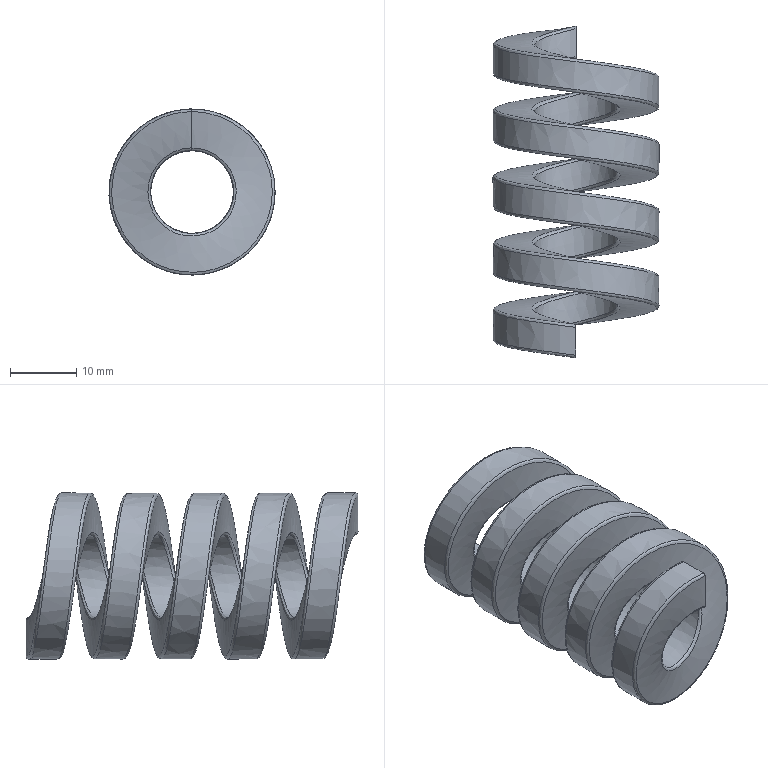Part | STEP file | solid 35 | 1 solid | 10 faces | box 25.029 x 50 x 25.037 mm | volume 8248 mm3 | spline 8 | plane 2